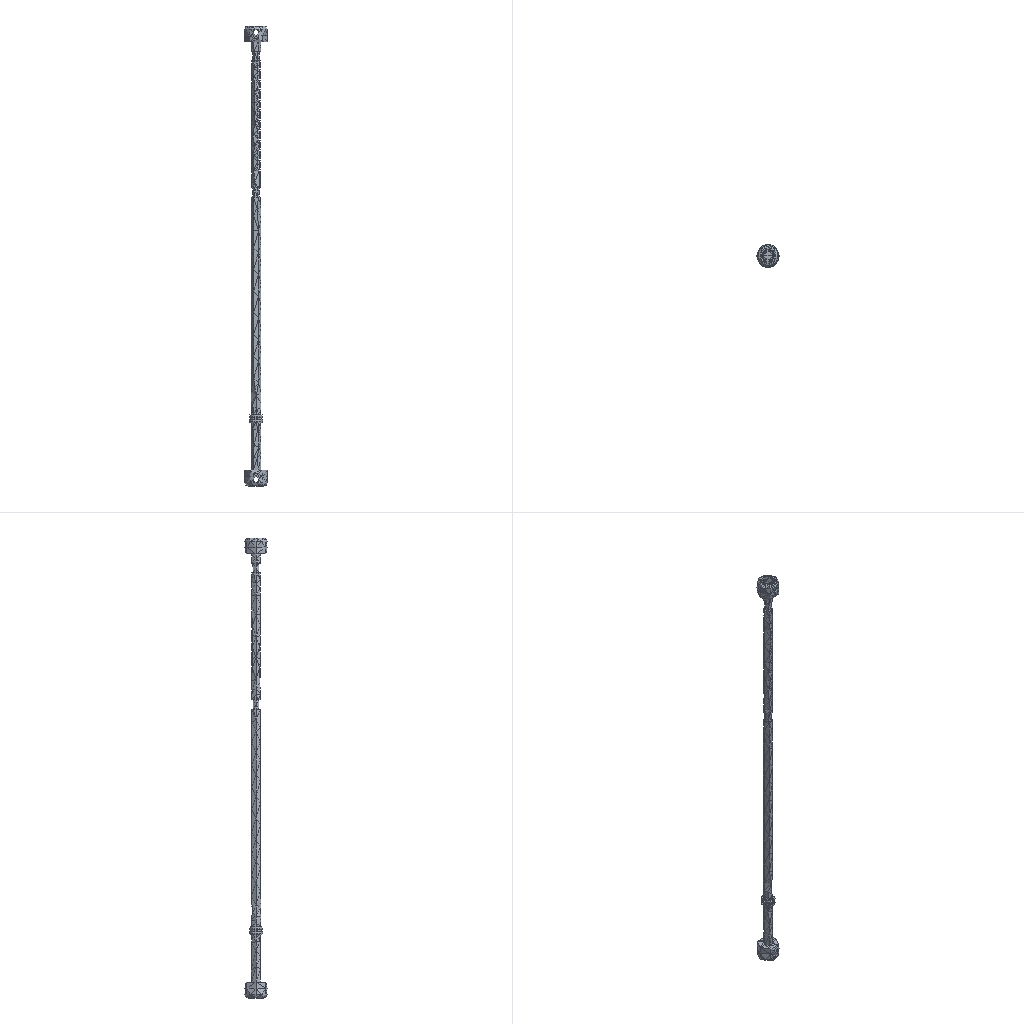Simulation study | ansys workbench
Ansys APDL input file, long lists of numbers shortened:
/batch
/config,noeldb,1     ! force off writing results to database
*get,_wallstrt,active,,time,wall
! ANSYS input file written by Workbench version 2022 R1
! File used for geometry attach: F:\ansys（分析文件汇总)\ansys转向器有限元分析\转向器\分析\啮合分析.STEP
/title,wbnew--____ (K5)
! ****** Begin Custom Load Command Snippet ******
/COM, ACT Extensions:
/COM,     LSDYNA, 2021.1
/COM,
! ****** End   Custom Load Command Snippet ******
*DIM,_wb_ProjectScratch_dir,string,248
_wb_ProjectScratch_dir(1) = 'C:\Users\Administrator\AppData\Local\Temp\WB_Administrator_18756_2\_ProjectScratch\Scr021B\'
*DIM,_wb_SolverFiles_dir,string,248
_wb_SolverFiles_dir(1) = 'C:\Users\Administrator\AppData\Local\Temp\WB_Administrator_18756_2\wbnew_files\dp0\SYS-3\MECH\'
*DIM,_wb_userfiles_dir,string,248
_wb_userfiles_dir(1) = 'C:\Users\Administrator\AppData\Local\Temp\WB_Administrator_18756_2\wbnew_files\user_files\'
/com,--- Data in consistent NMM units. See Solving Units in the help system for more information.
/units,MPA
/nopr
/wb,file,start              !  signify a WB generated input file
/prep7
! Turn off shape checking because checks already performed inside WB mesher.
! See help system for more information.
SHPP,OFF,,NOWARN
/nolist
etcon,set             ! allow ANSYS to choose best KEYOP's for 180x elements, resets any applicable keyopt to MAPDL defaults
/com,*********** Nodes for the whole assembly ***********
nblock,3,,16405
(1i9,3e20.9e3)
        1    -2.264268356E+02    -1.372275985E+03     8.117618442E+02
! (14913 more lines like these left out)
-1
/com,*********** Nodes for all Remote Points ***********
nblock,3
(1i9,3e20.9e3)
    14915     1.374619274E+01    -1.422396083E+03     8.203972876E+02
-1
/wb,elem,start            !  set before creation of elements
/com,*********** Elements for Body 1 "___|__-__1" ***********
et,1,187
eblock,19,solid,,3773
(19i9)
        1        1        1        1        0        0        0        0       10        0     3598     8021     8032     8813     8796    11877    11986    11885    11884
! (7545 more lines like these left out)
-1
/com,*********** Elements for Body 2 "__|__-__4" ***********
et,2,187
eblock,19,solid,,3597
(19i9)
        2        2        2        2        0        0        0        0       10        0        1      112      673     1373     1356     2140     5603     2149     2148
! (7193 more lines like these left out)
-1
/wb,elem,end               !  done creating elements
/com,*********** Send User Defined Coordinate System(s) ***********
csys,0
toffst,273.15,  ! Temperature offset from absolute zero
/com,*********** Set Reference Temperature ***********
tref,22.
/wb,mat,start              !  starting to send materials
/com,*********** Send Materials ***********
Temperature = 'TEMP' ! Temperature
MP,DENS,1,7.85e-09,	! tonne mm^-3
MP,ALPX,1,1.2e-05,	! C^-1
MP,C,1,434000000,	! mm^2 s^-2 C^-1
MP,KXX,1,60.5,	! tonne mm s^-3 C^-1
MP,RSVX,1,0.00017,	! ohm mm
MP,EX,1,200000,	! tonne s^-2 mm^-1
MP,NUXY,1,0.3,
MP,MURX,1,10000,
Temperature = 'TEMP' ! Temperature
MP,DENS,2,7.85e-09,	! tonne mm^-3
MP,ALPX,2,1.2e-05,	! C^-1
MP,C,2,434000000,	! mm^2 s^-2 C^-1
MP,KXX,2,60.5,	! tonne mm s^-3 C^-1
MP,RSVX,2,0.00017,	! ohm mm
MP,EX,2,200000,	! tonne s^-2 mm^-1
MP,NUXY,2,0.3,
MP,MURX,2,10000,
/wb,mat,end                !  done sending materials
!************************* Model Summary ********************
!___|__-__1,	结构钢,	matid,	1
!__|__-__4,	结构钢,	matid,	2
!************************* End Model Summary ********************
! get the diagonal of the bounding box. Needed later for other things
*get,_xmin,node,,mnloc,x
*get,_ymin,node,,mnloc,y
*get,_zmin,node,,mnloc,z
*get,_xmax,node,,mxloc,x
*get,_ymax,node,,mxloc,y
*get,_zmax,node,,mxloc,z
_ASMDIAG=(_xmax-_xmin)*(_xmax-_xmin)+(_ymax-_ymin)*(_ymax-_ymin)+(_zmax-_zmin)*(_zmax-_zmin)
_ASMDIAG=SQRT(_ASMDIAG)
/wb,contact,start          !  starting to send contact
/com,*********** Create Contact "接触区域" ***********
/com,            Real Constant Set For Above Contact Is 4 & 3
*set,tid,4
*set,cid,3
r,tid
r,cid
et,tid,170
et,cid,174
eblock,10,,,40
(15i9)
    12104        4        4        4        0     7878     8389     8393     8393    10508    13517     8393    10509
! (39 more lines like these left out)
-1
eblock,10,,,40
(15i9)
    12144        3        3        3        0     7878     8389     8393     8393    10508    13517     8393    10509
! (39 more lines like these left out)
-1
eblock,10,,,70
(15i9)
    12184        3        4        3        0      286      287      750      750     3306     3310      750     3307
! (69 more lines like these left out)
-1
eblock,10,,,70
(15i9)
    12254        4        3        4        0      286      287      750      750     3306     3310      750     3307
! (69 more lines like these left out)
-1
keyo,cid,8,2               ! auto create asymmetric contact (from Program Controlled setting)
keyo,cid,10,0              ! adjust contact stiffness each NR iteration (from Program Controlled setting)
keyo,cid,12,5              ! bonded always
keyo,cid,18,1              ! small sliding turned on by application
keyo,cid,2,0               ! augmented Lagrange (from Program Controlled setting)
keyo,cid,4,0               ! on Gauss point (from Program Controlled setting)
keyo,cid,9,1               ! ignore initial gaps/penetration
keyo,cid,7,0               ! No Prediction
rmod,tid,3,10.      ! FKN
rmod,tid,5,0.       ! ICONT
rmod,tid,6,0.       ! PINB
rmod,tid,10,0.      ! CNOF
rmod,tid,12,0.      ! FKT
rmod,tid,36,29      ! WB DSID
rmod,cid,3,10.      ! FKN
rmod,cid,5,0.       ! ICONT
rmod,cid,6,0.       ! PINB
rmod,cid,10,0.      ! CNOF
rmod,cid,12,0.      ! FKT
rmod,cid,36,29      ! WB DSID
nsel,all
esel,all
/wb,contact,end            !  done creating contacts
/com,*********** Send Named Selection as Node Component ***********
CMBLOCK,______  ,NODE,     2928
(8i10)
       207       208       211       212       215       216       219       220
! (365 more lines like these left out)
/golist
/wb,load,start             !  starting to send loads
/com,*********** Fixed Supports ***********
CMBLOCK,_FIXEDSU,NODE,      445
(8i10)
        67        68        69        70        71        72        73        74
! (55 more lines like these left out)
cmsel,s,_FIXEDSU
d,all,all
nsel,all
/com,*********** Create Remote Point "内部远程点" ***********
! -------- Remote Point Used by "力矩" --------
*set,tid,6
*set,cid,5
et,cid,174
et,tid,170
keyo,tid,2,1               ! Don't fix the pilot node
keyo,tid,4,111111
keyo,cid,12,5              ! Bonded Contact
keyo,cid,4,1               ! Deformable RBE3 style load
keyo,cid,2,2               ! MPC style contact
eblock,10,,,886
(15i9)
    12324        5        5        5        0     7847     8081     8284     8284    10205    12150     8284    10206
! (885 more lines like these left out)
-1
*set,_npilot,14915
_npilot45=_npilot
type,tid
mat ,cid
real,cid
tshape,pilo
en,13210,_npilot
tshape
/com,*********** Construct Moment Using Remote Attachment ***********
/gst,on,on
fini
*get,_numnode,node,0,count
*get,_numelem,elem,0,count
*get, _MAXELEMNUM, elem, 0, NUM, MAX
*get, _MAXNODENUM, node, 0, NUM, MAX
*get, _MAXELEMTYPE, etyp, 0, NUM, MAX
*get, _MAXREALCONST, real, 0, NUM, MAX
/go
/wb,load,end               !  done creating loads
/com,--- Number of total nodes = %_numnode%
/com,--- Number of contact elements = 1106
/com,--- Number of spring elements = 0
/com,--- Number of bearing elements = 0
/com,--- Number of solid elements = 7370
/com,--- Number of condensed parts = 0
/com,--- Number of total elements = %_numelem%
*get,_wallbsol,active,,time,wall
/com,****************************************************************************
/com,*************************    SOLUTION       ********************************
/com,****************************************************************************
/solu
antype,0                   ! static analysis
_thickRatio=0.5     ! Ratio of thick parts in the model
eqsl,sparse,,,,,1
cntr,print,1               ! print out contact info and also make no initial contact an error
dmpoption,emat,no             ! Don't combine emat file for DANSYS
dmpoption,esav,no             ! Don't combine esav file for DANSYS
nldiag,cont,iter           ! print out contact info each equilibrium iteration
rescontrol,,none                 ! Do not keep any restart files
/com,****************************************************
/com,******************* SOLVE FOR LS 1 OF 1 ****************
nsel,s,node,,14915
f,all,mx,0.
f,all,my,500000.
f,all,mz,0.
nsel,all
/nopr
/gopr
nsub,1,1,1
time,1.
outres,erase
outres,all,none
outres,nsol,all,
outres,rsol,all
outres,eangl,all
outres,etmp,all
outres,veng,all
outres,strs,all,
outres,epel,all,
outres,eppl,all,
outres,cont,all,
! *********** WB SOLVE COMMAND ***********
! check interactive state
*get,ANSINTER_,active,,int
*if,ANSINTER_,ne,0,then
/eof
*endif
solve
/com *************** Write FE CONNECTORS *********
CEWRITE,file,ce,,INTE
/com,****************************************************
/com,*************** FINISHED SOLVE FOR LS 1 *************
*get,_wallasol,active,,time,wall
/nopr
*get,_numnode,node,0,count
*get,_numelem,elem,0,count
*get, _MAXELEMNUM, elem, 0, NUM, MAX
*get, _MAXNODENUM, node, 0, NUM, MAX,,,INTERNAL
*get, _MAXELEMTYPE, etyp, 0, NUM, MAX
*get, _MAXREALCONST, real, 0, NUM, MAX
/gopr
/post1
xmlo,ENCODING,ISO-8859-1
xmlo,parm
/xml,parm,xml
fini
/gopr
*get,_walldone,active,,time,wall
_preptime=(_wallbsol-_wallstrt)*3600
_solvtime=(_wallasol-_wallbsol)*3600
_posttime=(_walldone-_wallasol)*3600
_totaltim=(_walldone-_wallstrt)*3600
*get,_dlbratio,active,0,solu,dlbr
*get,_combtime,active,0,solu,comb
*get,_ssmode,active,0,solu,ssmm
*get,_ndofs,active,0,solu,ndof
*get,_sol_end_time,active,0,set,time
*if,_sol_end_time,eq,1.,then
/fclean				!clean distributed files
*endif
/com,--- Total number of nodes = %_numnode%
/com,--- Total number of elements = %_numelem%
/com,--- Element load balance ratio = %_dlbratio%
/com,--- Time to combine distributed files = %_combtime%
/com,--- Sparse memory mode = %_ssmode%
/com,--- Number of DOF = %_ndofs%
/wb,file,end               ! done with WB generated input